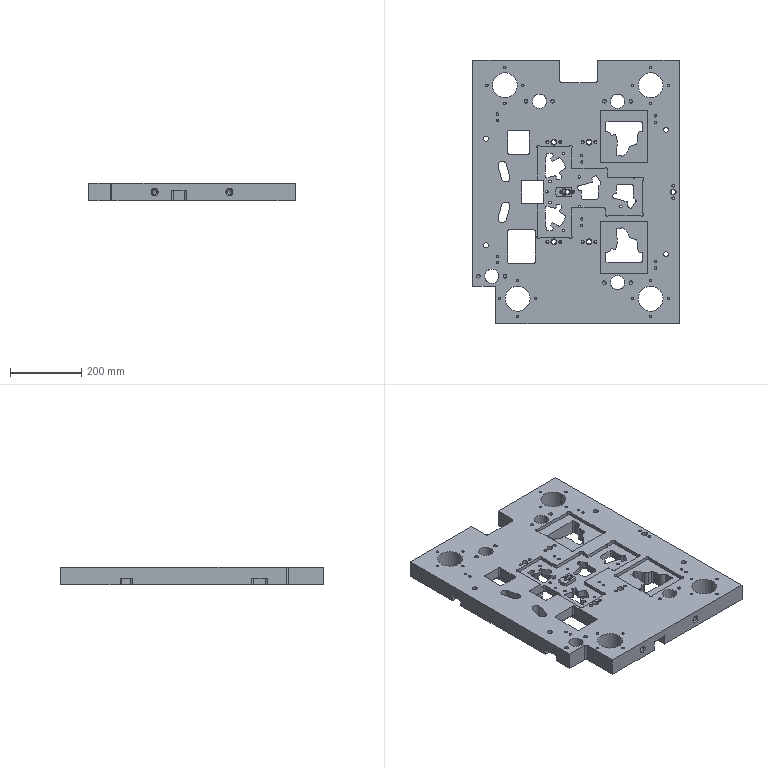Part | NX | features solid 2 | 1 solid | 552 faces | box 580 x 740 x 50 mm | volume 15717918 mm3 | cylinder 274 | plane 202 | cone 52 | spline 24 | commonest cylinder face diameters 6.8 x48 8 x48 10 x42 6 x18 5 x12 8.5 x12